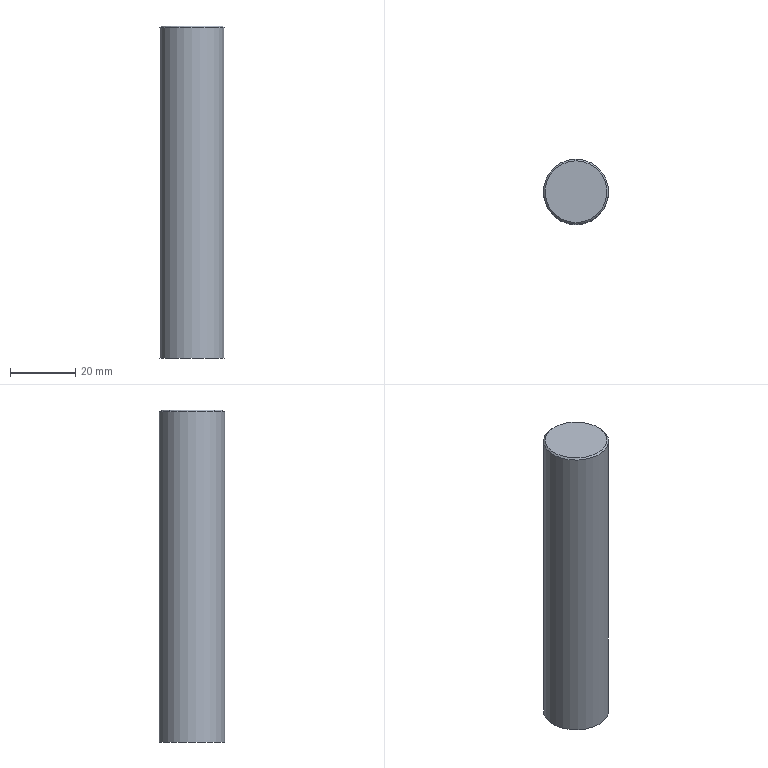Part | NX | features solid 2 | 1 solid | 4 faces | box 20 x 20 x 102 mm | volume 32037 mm3 | plane 2 | cylinder 1 | cone 1 | commonest cylinder face diameters 20 x1
STEP:
#1=CARTESIAN_POINT('',(200.,-80.,-87.5));
#2=VERTEX_POINT('',#1);
#3=CARTESIAN_POINT('',(200.,-90.,-87.5));
#4=DIRECTION('',(0.,0.,-1.));
#5=DIRECTION('',(0.,1.,0.));
#6=AXIS2_PLACEMENT_3D('',#3,#4,#5);
#7=CIRCLE('',#6,10.);
#8=EDGE_CURVE('',#2,#2,#7,.T.);
#9=ORIENTED_EDGE('',*,*,#8,.T.);
#10=EDGE_LOOP('',(#9));
#11=FACE_BOUND('',#10,.T.);
#12=CARTESIAN_POINT('',(200.,-80.,-189.));
#13=VERTEX_POINT('',#12);
#14=CARTESIAN_POINT('',(200.,-90.,-189.));
#15=DIRECTION('',(0.,0.,-1.));
#16=DIRECTION('',(0.,1.,0.));
#17=AXIS2_PLACEMENT_3D('',#14,#15,#16);
#18=CIRCLE('',#17,10.);
#19=EDGE_CURVE('',#13,#13,#18,.T.);
#20=ORIENTED_EDGE('',*,*,#19,.F.);
#21=EDGE_LOOP('',(#20));
#22=FACE_BOUND('',#21,.T.);
#23=CARTESIAN_POINT('',(200.,-90.,-189.));
#24=DIRECTION('',(0.,0.,1.));
#25=DIRECTION('',(0.,-1.,0.));
#26=AXIS2_PLACEMENT_3D('',#23,#24,#25);
#27=CYLINDRICAL_SURFACE('',#26,10.);
#28=ADVANCED_FACE('',(#11,#22),#27,.T.);
#29=ORIENTED_EDGE('',*,*,#19,.T.);
#30=EDGE_LOOP('',(#29));
#31=FACE_BOUND('',#30,.T.);
#32=CARTESIAN_POINT('',(200.,-90.,-189.));
#33=DIRECTION('',(0.,0.,-1.));
#34=DIRECTION('',(0.,1.,0.));
#35=AXIS2_PLACEMENT_3D('',#32,#33,#34);
#36=PLANE('',#35);
#37=ADVANCED_FACE('',(#31),#36,.T.);
#38=CARTESIAN_POINT('',(200.,-80.5,-87.));
#39=VERTEX_POINT('',#38);
#40=CARTESIAN_POINT('',(200.,-90.,-87.));
#41=DIRECTION('',(0.,0.,-1.));
#42=DIRECTION('',(0.,1.,0.));
#43=AXIS2_PLACEMENT_3D('',#40,#41,#42);
#44=CIRCLE('',#43,9.5);
#45=EDGE_CURVE('',#39,#39,#44,.F.);
#46=ORIENTED_EDGE('',*,*,#45,.T.);
#47=EDGE_LOOP('',(#46));
#48=FACE_BOUND('',#47,.T.);
#49=CARTESIAN_POINT('',(200.,-90.,-87.));
#50=DIRECTION('',(0.,0.,-1.));
#51=DIRECTION('',(0.,1.,0.));
#52=AXIS2_PLACEMENT_3D('',#49,#50,#51);
#53=PLANE('',#52);
#54=ADVANCED_FACE('',(#48),#53,.F.);
#55=ORIENTED_EDGE('',*,*,#45,.F.);
#56=EDGE_LOOP('',(#55));
#57=FACE_BOUND('',#56,.T.);
#58=ORIENTED_EDGE('',*,*,#8,.F.);
#59=EDGE_LOOP('',(#58));
#60=FACE_BOUND('',#59,.T.);
#61=CARTESIAN_POINT('',(200.,-90.,-87.5));
#62=DIRECTION('',(0.,0.,-1.));
#63=DIRECTION('',(0.,1.,0.));
#64=AXIS2_PLACEMENT_3D('',#61,#62,#63);
#65=CONICAL_SURFACE('',#64,10.,0.7854);
#66=ADVANCED_FACE('',(#57,#60),#65,.T.);
#67=CLOSED_SHELL('',(#28,#37,#54,#66));
#68=MANIFOLD_SOLID_BREP('',#67);
#69=(LENGTH_UNIT()NAMED_UNIT(*)SI_UNIT(.MILLI.,.METRE.));
#70=UNCERTAINTY_MEASURE_WITH_UNIT(LENGTH_MEASURE(0.00001),#69,'','');
#71=(NAMED_UNIT(*)PLANE_ANGLE_UNIT()SI_UNIT($,.RADIAN.));
#72=(NAMED_UNIT(*)SI_UNIT($,.STERADIAN.)SOLID_ANGLE_UNIT());
#73=(GEOMETRIC_REPRESENTATION_CONTEXT(3)GLOBAL_UNCERTAINTY_ASSIGNED_CONTEXT((#70))GLOBAL_UNIT_ASSIGNED_CONTEXT((#69,#71,#72))REPRESENTATION_CONTEXT('',''));
#74=ADVANCED_BREP_SHAPE_REPRESENTATION('',(#68),#73);